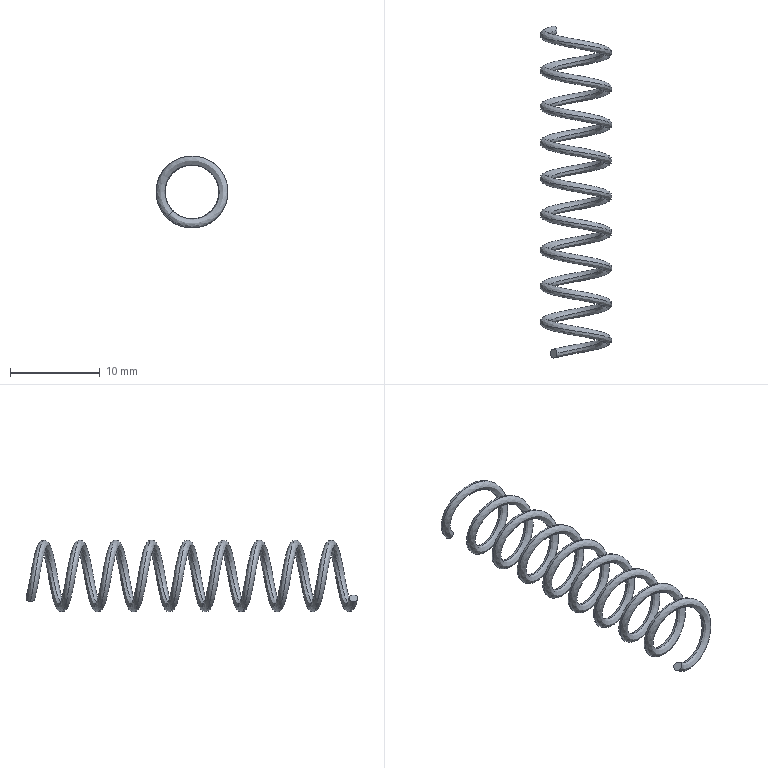Part | STEP file | BCC3 H14_10 | 1 solid | 4 faces | box 8 x 37 x 8 mm | volume 155.461 mm3 | spline 2 | plane 2